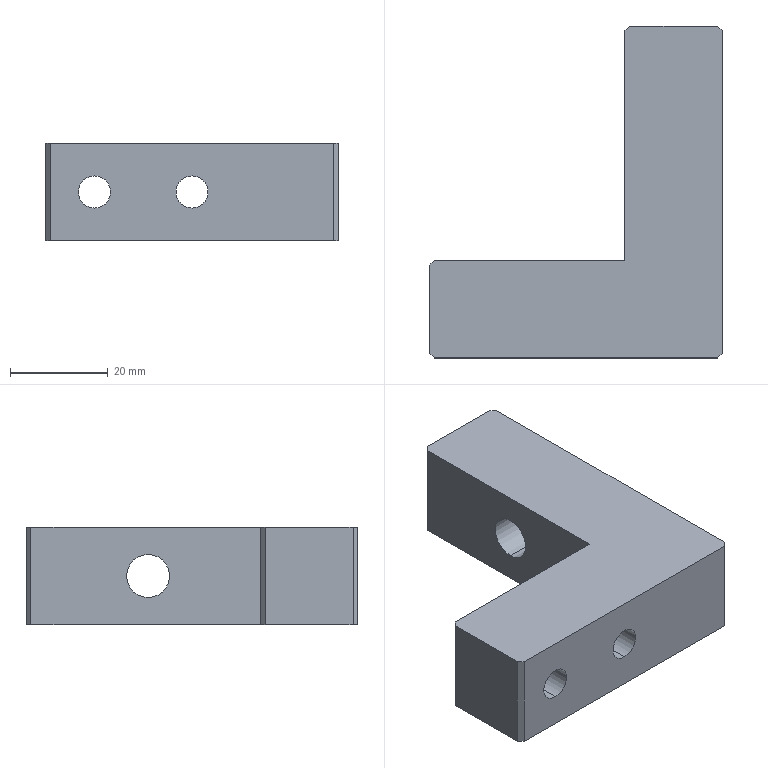Part | SolidWorks | features HoleWzd 2, Chamfer 1, Extrusion 1 | 1 solid | 25 faces | box 60 x 68 x 20 mm | volume 39349 mm3 | plane 15 | cylinder 10 | commonest cylinder face diameters 6.6 x4 11 x4 8.8 x2
STEP:
#1=CARTESIAN_POINT('',(-3.564,-15.126,4.5));
#2=VERTEX_POINT('',#1);
#3=CARTESIAN_POINT('',(-3.564,-15.126,15.5));
#4=VERTEX_POINT('',#3);
#5=CARTESIAN_POINT('',(-3.564,-15.126,10.));
#6=DIRECTION('',(0.,1.,0.));
#7=DIRECTION('',(0.,0.,1.));
#8=AXIS2_PLACEMENT_3D('',#5,#6,#7);
#9=CIRCLE('',#8,5.5);
#10=EDGE_CURVE('',#2,#4,#9,.T.);
#11=ORIENTED_EDGE('',*,*,#10,.F.);
#12=CARTESIAN_POINT('',(-3.564,-5.126,4.5));
#13=VERTEX_POINT('',#12);
#14=CARTESIAN_POINT('',(-3.564,-5.126,4.5));
#15=DIRECTION('',(0.,1.,0.));
#16=VECTOR('',#15,1000.);
#17=LINE('',#14,#16);
#18=EDGE_CURVE('',#2,#13,#17,.T.);
#19=ORIENTED_EDGE('',*,*,#18,.T.);
#20=CARTESIAN_POINT('',(-3.564,-5.126,15.5));
#21=VERTEX_POINT('',#20);
#22=CARTESIAN_POINT('',(-3.564,-5.126,10.));
#23=DIRECTION('',(0.,1.,0.));
#24=DIRECTION('',(0.,0.,1.));
#25=AXIS2_PLACEMENT_3D('',#22,#23,#24);
#26=CIRCLE('',#25,5.5);
#27=EDGE_CURVE('',#13,#21,#26,.T.);
#28=ORIENTED_EDGE('',*,*,#27,.T.);
#29=CARTESIAN_POINT('',(-3.564,-5.126,15.5));
#30=DIRECTION('',(0.,1.,0.));
#31=VECTOR('',#30,1000.);
#32=LINE('',#29,#31);
#33=EDGE_CURVE('',#4,#21,#32,.T.);
#34=ORIENTED_EDGE('',*,*,#33,.F.);
#35=EDGE_LOOP('',(#11,#19,#28,#34));
#36=FACE_OUTER_BOUND('',#35,.T.);
#37=CARTESIAN_POINT('',(-3.564,-5.126,10.));
#38=DIRECTION('',(0.,1.,0.));
#39=DIRECTION('',(0.,0.,1.));
#40=AXIS2_PLACEMENT_3D('',#37,#38,#39);
#41=CYLINDRICAL_SURFACE('',#40,5.5);
#42=ADVANCED_FACE('',(#36),#41,.F.);
#43=CARTESIAN_POINT('',(-3.564,-25.126,6.7));
#44=VERTEX_POINT('',#43);
#45=CARTESIAN_POINT('',(-3.564,-25.126,13.3));
#46=VERTEX_POINT('',#45);
#47=CARTESIAN_POINT('',(-3.564,-25.126,10.));
#48=DIRECTION('',(0.,1.,0.));
#49=DIRECTION('',(0.,0.,1.));
#50=AXIS2_PLACEMENT_3D('',#47,#48,#49);
#51=CIRCLE('',#50,3.3);
#52=EDGE_CURVE('',#44,#46,#51,.T.);
#53=ORIENTED_EDGE('',*,*,#52,.F.);
#54=CARTESIAN_POINT('',(-3.564,-15.126,6.7));
#55=VERTEX_POINT('',#54);
#56=CARTESIAN_POINT('',(-3.564,-5.126,6.7));
#57=DIRECTION('',(0.,1.,0.));
#58=VECTOR('',#57,1000.);
#59=LINE('',#56,#58);
#60=EDGE_CURVE('',#44,#55,#59,.T.);
#61=ORIENTED_EDGE('',*,*,#60,.T.);
#62=CARTESIAN_POINT('',(-3.564,-15.126,13.3));
#63=VERTEX_POINT('',#62);
#64=CARTESIAN_POINT('',(-3.564,-15.126,10.));
#65=DIRECTION('',(0.,1.,0.));
#66=DIRECTION('',(0.,0.,1.));
#67=AXIS2_PLACEMENT_3D('',#64,#65,#66);
#68=CIRCLE('',#67,3.3);
#69=EDGE_CURVE('',#55,#63,#68,.T.);
#70=ORIENTED_EDGE('',*,*,#69,.T.);
#71=CARTESIAN_POINT('',(-3.564,-5.126,13.3));
#72=DIRECTION('',(0.,1.,0.));
#73=VECTOR('',#72,1000.);
#74=LINE('',#71,#73);
#75=EDGE_CURVE('',#46,#63,#74,.T.);
#76=ORIENTED_EDGE('',*,*,#75,.F.);
#77=EDGE_LOOP('',(#53,#61,#70,#76));
#78=FACE_OUTER_BOUND('',#77,.T.);
#79=CARTESIAN_POINT('',(-3.564,-5.126,10.));
#80=DIRECTION('',(0.,1.,0.));
#81=DIRECTION('',(0.,0.,1.));
#82=AXIS2_PLACEMENT_3D('',#79,#80,#81);
#83=CYLINDRICAL_SURFACE('',#82,3.3);
#84=ADVANCED_FACE('',(#78),#83,.F.);
#85=CARTESIAN_POINT('',(-23.564,-15.126,4.5));
#86=VERTEX_POINT('',#85);
#87=CARTESIAN_POINT('',(-23.564,-15.126,15.5));
#88=VERTEX_POINT('',#87);
#89=CARTESIAN_POINT('',(-23.564,-15.126,10.));
#90=DIRECTION('',(0.,1.,0.));
#91=DIRECTION('',(0.,0.,1.));
#92=AXIS2_PLACEMENT_3D('',#89,#90,#91);
#93=CIRCLE('',#92,5.5);
#94=EDGE_CURVE('',#86,#88,#93,.T.);
#95=ORIENTED_EDGE('',*,*,#94,.F.);
#96=CARTESIAN_POINT('',(-23.564,-5.126,4.5));
#97=VERTEX_POINT('',#96);
#98=CARTESIAN_POINT('',(-23.564,-5.126,4.5));
#99=DIRECTION('',(0.,1.,0.));
#100=VECTOR('',#99,1000.);
#101=LINE('',#98,#100);
#102=EDGE_CURVE('',#86,#97,#101,.T.);
#103=ORIENTED_EDGE('',*,*,#102,.T.);
#104=CARTESIAN_POINT('',(-23.564,-5.126,15.5));
#105=VERTEX_POINT('',#104);
#106=CARTESIAN_POINT('',(-23.564,-5.126,10.));
#107=DIRECTION('',(0.,1.,0.));
#108=DIRECTION('',(0.,0.,1.));
#109=AXIS2_PLACEMENT_3D('',#106,#107,#108);
#110=CIRCLE('',#109,5.5);
#111=EDGE_CURVE('',#97,#105,#110,.T.);
#112=ORIENTED_EDGE('',*,*,#111,.T.);
#113=CARTESIAN_POINT('',(-23.564,-5.126,15.5));
#114=DIRECTION('',(0.,1.,0.));
#115=VECTOR('',#114,1000.);
#116=LINE('',#113,#115);
#117=EDGE_CURVE('',#88,#105,#116,.T.);
#118=ORIENTED_EDGE('',*,*,#117,.F.);
#119=EDGE_LOOP('',(#95,#103,#112,#118));
#120=FACE_OUTER_BOUND('',#119,.T.);
#121=CARTESIAN_POINT('',(-23.564,-5.126,10.));
#122=DIRECTION('',(0.,1.,0.));
#123=DIRECTION('',(0.,0.,1.));
#124=AXIS2_PLACEMENT_3D('',#121,#122,#123);
#125=CYLINDRICAL_SURFACE('',#124,5.5);
#126=ADVANCED_FACE('',(#120),#125,.F.);
#127=CARTESIAN_POINT('',(-23.564,-25.126,6.7));
#128=VERTEX_POINT('',#127);
#129=CARTESIAN_POINT('',(-23.564,-25.126,13.3));
#130=VERTEX_POINT('',#129);
#131=CARTESIAN_POINT('',(-23.564,-25.126,10.));
#132=DIRECTION('',(0.,1.,0.));
#133=DIRECTION('',(0.,0.,1.));
#134=AXIS2_PLACEMENT_3D('',#131,#132,#133);
#135=CIRCLE('',#134,3.3);
#136=EDGE_CURVE('',#128,#130,#135,.T.);
#137=ORIENTED_EDGE('',*,*,#136,.F.);
#138=CARTESIAN_POINT('',(-23.564,-15.126,6.7));
#139=VERTEX_POINT('',#138);
#140=CARTESIAN_POINT('',(-23.564,-5.126,6.7));
#141=DIRECTION('',(0.,1.,0.));
#142=VECTOR('',#141,1000.);
#143=LINE('',#140,#142);
#144=EDGE_CURVE('',#128,#139,#143,.T.);
#145=ORIENTED_EDGE('',*,*,#144,.T.);
#146=CARTESIAN_POINT('',(-23.564,-15.126,13.3));
#147=VERTEX_POINT('',#146);
#148=CARTESIAN_POINT('',(-23.564,-15.126,10.));
#149=DIRECTION('',(0.,1.,0.));
#150=DIRECTION('',(0.,0.,1.));
#151=AXIS2_PLACEMENT_3D('',#148,#149,#150);
#152=CIRCLE('',#151,3.3);
#153=EDGE_CURVE('',#139,#147,#152,.T.);
#154=ORIENTED_EDGE('',*,*,#153,.T.);
#155=CARTESIAN_POINT('',(-23.564,-5.126,13.3));
#156=DIRECTION('',(0.,1.,0.));
#157=VECTOR('',#156,1000.);
#158=LINE('',#155,#157);
#159=EDGE_CURVE('',#130,#147,#158,.T.);
#160=ORIENTED_EDGE('',*,*,#159,.F.);
#161=EDGE_LOOP('',(#137,#145,#154,#160));
#162=FACE_OUTER_BOUND('',#161,.T.);
#163=CARTESIAN_POINT('',(-23.564,-5.126,10.));
#164=DIRECTION('',(0.,1.,0.));
#165=DIRECTION('',(0.,0.,1.));
#166=AXIS2_PLACEMENT_3D('',#163,#164,#165);
#167=CYLINDRICAL_SURFACE('',#166,3.3);
#168=ADVANCED_FACE('',(#162),#167,.F.);
#169=CARTESIAN_POINT('',(26.436,17.874,5.6));
#170=VERTEX_POINT('',#169);
#171=CARTESIAN_POINT('',(26.436,17.874,14.4));
#172=VERTEX_POINT('',#171);
#173=CARTESIAN_POINT('',(26.436,17.874,10.));
#174=DIRECTION('',(-1.,0.,0.));
#175=DIRECTION('',(0.,0.,1.));
#176=AXIS2_PLACEMENT_3D('',#173,#174,#175);
#177=CIRCLE('',#176,4.4);
#178=EDGE_CURVE('',#170,#172,#177,.T.);
#179=ORIENTED_EDGE('',*,*,#178,.F.);
#180=CARTESIAN_POINT('',(6.436,17.874,5.6));
#181=VERTEX_POINT('',#180);
#182=CARTESIAN_POINT('',(6.436,17.874,5.6));
#183=DIRECTION('',(-1.,0.,0.));
#184=VECTOR('',#183,1000.);
#185=LINE('',#182,#184);
#186=EDGE_CURVE('',#170,#181,#185,.T.);
#187=ORIENTED_EDGE('',*,*,#186,.T.);
#188=CARTESIAN_POINT('',(6.436,17.874,14.4));
#189=VERTEX_POINT('',#188);
#190=CARTESIAN_POINT('',(6.436,17.874,10.));
#191=DIRECTION('',(-1.,0.,0.));
#192=DIRECTION('',(0.,0.,1.));
#193=AXIS2_PLACEMENT_3D('',#190,#191,#192);
#194=CIRCLE('',#193,4.4);
#195=EDGE_CURVE('',#181,#189,#194,.T.);
#196=ORIENTED_EDGE('',*,*,#195,.T.);
#197=CARTESIAN_POINT('',(6.436,17.874,14.4));
#198=DIRECTION('',(-1.,0.,0.));
#199=VECTOR('',#198,1000.);
#200=LINE('',#197,#199);
#201=EDGE_CURVE('',#172,#189,#200,.T.);
#202=ORIENTED_EDGE('',*,*,#201,.F.);
#203=EDGE_LOOP('',(#179,#187,#196,#202));
#204=FACE_OUTER_BOUND('',#203,.T.);
#205=CARTESIAN_POINT('',(6.436,17.874,10.));
#206=DIRECTION('',(-1.,0.,0.));
#207=DIRECTION('',(0.,0.,1.));
#208=AXIS2_PLACEMENT_3D('',#205,#206,#207);
#209=CYLINDRICAL_SURFACE('',#208,4.4);
#210=ADVANCED_FACE('',(#204),#209,.F.);
#211=CARTESIAN_POINT('',(25.436,42.874,0.));
#212=VERTEX_POINT('',#211);
#213=CARTESIAN_POINT('',(7.436,42.874,0.));
#214=VERTEX_POINT('',#213);
#215=CARTESIAN_POINT('',(26.436,42.874,0.));
#216=DIRECTION('',(-1.,0.,0.));
#217=VECTOR('',#216,1000.);
#218=LINE('',#215,#217);
#219=EDGE_CURVE('',#212,#214,#218,.T.);
#220=ORIENTED_EDGE('',*,*,#219,.T.);
#221=CARTESIAN_POINT('',(7.436,42.874,20.));
#222=VERTEX_POINT('',#221);
#223=CARTESIAN_POINT('',(7.436,42.874,20.));
#224=DIRECTION('',(0.,0.,1.));
#225=VECTOR('',#224,1000.);
#226=LINE('',#223,#225);
#227=EDGE_CURVE('',#214,#222,#226,.T.);
#228=ORIENTED_EDGE('',*,*,#227,.T.);
#229=CARTESIAN_POINT('',(25.436,42.874,20.));
#230=VERTEX_POINT('',#229);
#231=CARTESIAN_POINT('',(26.436,42.874,20.));
#232=DIRECTION('',(-1.,0.,0.));
#233=VECTOR('',#232,1000.);
#234=LINE('',#231,#233);
#235=EDGE_CURVE('',#230,#222,#234,.T.);
#236=ORIENTED_EDGE('',*,*,#235,.F.);
#237=CARTESIAN_POINT('',(25.436,42.874,20.));
#238=DIRECTION('',(0.,0.,-1.));
#239=VECTOR('',#238,1000.);
#240=LINE('',#237,#239);
#241=EDGE_CURVE('',#230,#212,#240,.T.);
#242=ORIENTED_EDGE('',*,*,#241,.T.);
#243=EDGE_LOOP('',(#220,#228,#236,#242));
#244=FACE_OUTER_BOUND('',#243,.T.);
#245=CARTESIAN_POINT('',(26.436,42.874,20.));
#246=DIRECTION('',(0.,-1.,0.));
#247=DIRECTION('',(0.,0.,-1.));
#248=AXIS2_PLACEMENT_3D('',#245,#246,#247);
#249=PLANE('',#248);
#250=ADVANCED_FACE('',(#244),#249,.F.);
#251=CARTESIAN_POINT('',(6.436,17.874,10.));
#252=DIRECTION('',(-1.,0.,0.));
#253=DIRECTION('',(0.,0.,1.));
#254=AXIS2_PLACEMENT_3D('',#251,#252,#253);
#255=CIRCLE('',#254,4.4);
#256=EDGE_CURVE('',#189,#181,#255,.T.);
#257=ORIENTED_EDGE('',*,*,#256,.F.);
#258=ORIENTED_EDGE('',*,*,#195,.F.);
#259=EDGE_LOOP('',(#257,#258));
#260=FACE_BOUND('',#259,.T.);
#261=CARTESIAN_POINT('',(6.436,41.874,20.));
#262=VERTEX_POINT('',#261);
#263=CARTESIAN_POINT('',(6.436,-5.126,20.));
#264=VERTEX_POINT('',#263);
#265=CARTESIAN_POINT('',(6.436,42.874,20.));
#266=DIRECTION('',(0.,-1.,0.));
#267=VECTOR('',#266,1000.);
#268=LINE('',#265,#267);
#269=EDGE_CURVE('',#262,#264,#268,.T.);
#270=ORIENTED_EDGE('',*,*,#269,.F.);
#271=CARTESIAN_POINT('',(6.436,41.874,0.));
#272=VERTEX_POINT('',#271);
#273=CARTESIAN_POINT('',(6.436,41.874,20.));
#274=DIRECTION('',(0.,0.,-1.));
#275=VECTOR('',#274,1000.);
#276=LINE('',#273,#275);
#277=EDGE_CURVE('',#262,#272,#276,.T.);
#278=ORIENTED_EDGE('',*,*,#277,.T.);
#279=CARTESIAN_POINT('',(6.436,-5.126,0.));
#280=VERTEX_POINT('',#279);
#281=CARTESIAN_POINT('',(6.436,42.874,0.));
#282=DIRECTION('',(0.,-1.,0.));
#283=VECTOR('',#282,1000.);
#284=LINE('',#281,#283);
#285=EDGE_CURVE('',#272,#280,#284,.T.);
#286=ORIENTED_EDGE('',*,*,#285,.T.);
#287=CARTESIAN_POINT('',(6.436,-5.126,20.));
#288=DIRECTION('',(0.,0.,-1.));
#289=VECTOR('',#288,1000.);
#290=LINE('',#287,#289);
#291=EDGE_CURVE('',#264,#280,#290,.T.);
#292=ORIENTED_EDGE('',*,*,#291,.F.);
#293=EDGE_LOOP('',(#270,#278,#286,#292));
#294=FACE_OUTER_BOUND('',#293,.T.);
#295=CARTESIAN_POINT('',(6.436,42.874,20.));
#296=DIRECTION('',(1.,0.,0.));
#297=DIRECTION('',(0.,1.,0.));
#298=AXIS2_PLACEMENT_3D('',#295,#296,#297);
#299=PLANE('',#298);
#300=ADVANCED_FACE('',(#260,#294),#299,.F.);
#301=CARTESIAN_POINT('',(-3.564,-5.126,10.));
#302=DIRECTION('',(0.,1.,0.));
#303=DIRECTION('',(0.,0.,1.));
#304=AXIS2_PLACEMENT_3D('',#301,#302,#303);
#305=CIRCLE('',#304,5.5);
#306=EDGE_CURVE('',#21,#13,#305,.T.);
#307=ORIENTED_EDGE('',*,*,#306,.F.);
#308=ORIENTED_EDGE('',*,*,#27,.F.);
#309=EDGE_LOOP('',(#307,#308));
#310=FACE_BOUND('',#309,.T.);
#311=CARTESIAN_POINT('',(-23.564,-5.126,10.));
#312=DIRECTION('',(0.,1.,0.));
#313=DIRECTION('',(0.,0.,1.));
#314=AXIS2_PLACEMENT_3D('',#311,#312,#313);
#315=CIRCLE('',#314,5.5);
#316=EDGE_CURVE('',#105,#97,#315,.T.);
#317=ORIENTED_EDGE('',*,*,#316,.F.);
#318=ORIENTED_EDGE('',*,*,#111,.F.);
#319=EDGE_LOOP('',(#317,#318));
#320=FACE_BOUND('',#319,.T.);
#321=CARTESIAN_POINT('',(-32.564,-5.126,0.));
#322=VERTEX_POINT('',#321);
#323=CARTESIAN_POINT('',(6.436,-5.126,0.));
#324=DIRECTION('',(-1.,0.,0.));
#325=VECTOR('',#324,1000.);
#326=LINE('',#323,#325);
#327=EDGE_CURVE('',#280,#322,#326,.T.);
#328=ORIENTED_EDGE('',*,*,#327,.T.);
#329=CARTESIAN_POINT('',(-32.564,-5.126,20.));
#330=VERTEX_POINT('',#329);
#331=CARTESIAN_POINT('',(-32.564,-5.126,20.));
#332=DIRECTION('',(0.,0.,1.));
#333=VECTOR('',#332,1000.);
#334=LINE('',#331,#333);
#335=EDGE_CURVE('',#322,#330,#334,.T.);
#336=ORIENTED_EDGE('',*,*,#335,.T.);
#337=CARTESIAN_POINT('',(6.436,-5.126,20.));
#338=DIRECTION('',(-1.,0.,0.));
#339=VECTOR('',#338,1000.);
#340=LINE('',#337,#339);
#341=EDGE_CURVE('',#264,#330,#340,.T.);
#342=ORIENTED_EDGE('',*,*,#341,.F.);
#343=ORIENTED_EDGE('',*,*,#291,.T.);
#344=EDGE_LOOP('',(#328,#336,#342,#343));
#345=FACE_OUTER_BOUND('',#344,.T.);
#346=CARTESIAN_POINT('',(6.436,-5.126,20.));
#347=DIRECTION('',(0.,-1.,0.));
#348=DIRECTION('',(1.,0.,0.));
#349=AXIS2_PLACEMENT_3D('',#346,#347,#348);
#350=PLANE('',#349);
#351=ADVANCED_FACE('',(#310,#320,#345),#350,.F.);
#352=CARTESIAN_POINT('',(-33.564,-6.126,0.));
#353=VERTEX_POINT('',#352);
#354=CARTESIAN_POINT('',(-33.564,-24.126,0.));
#355=VERTEX_POINT('',#354);
#356=CARTESIAN_POINT('',(-33.564,-5.126,0.));
#357=DIRECTION('',(0.,-1.,0.));
#358=VECTOR('',#357,1000.);
#359=LINE('',#356,#358);
#360=EDGE_CURVE('',#353,#355,#359,.T.);
#361=ORIENTED_EDGE('',*,*,#360,.T.);
#362=CARTESIAN_POINT('',(-33.564,-24.126,20.));
#363=VERTEX_POINT('',#362);
#364=CARTESIAN_POINT('',(-33.564,-24.126,20.));
#365=DIRECTION('',(0.,0.,1.));
#366=VECTOR('',#365,1000.);
#367=LINE('',#364,#366);
#368=EDGE_CURVE('',#355,#363,#367,.T.);
#369=ORIENTED_EDGE('',*,*,#368,.T.);
#370=CARTESIAN_POINT('',(-33.564,-6.126,20.));
#371=VERTEX_POINT('',#370);
#372=CARTESIAN_POINT('',(-33.564,-5.126,20.));
#373=DIRECTION('',(0.,-1.,0.));
#374=VECTOR('',#373,1000.);
#375=LINE('',#372,#374);
#376=EDGE_CURVE('',#371,#363,#375,.T.);
#377=ORIENTED_EDGE('',*,*,#376,.F.);
#378=CARTESIAN_POINT('',(-33.564,-6.126,20.));
#379=DIRECTION('',(0.,0.,-1.));
#380=VECTOR('',#379,1000.);
#381=LINE('',#378,#380);
#382=EDGE_CURVE('',#371,#353,#381,.T.);
#383=ORIENTED_EDGE('',*,*,#382,.T.);
#384=EDGE_LOOP('',(#361,#369,#377,#383));
#385=FACE_OUTER_BOUND('',#384,.T.);
#386=CARTESIAN_POINT('',(-33.564,-5.126,20.));
#387=DIRECTION('',(1.,0.,0.));
#388=DIRECTION('',(0.,1.,0.));
#389=AXIS2_PLACEMENT_3D('',#386,#387,#388);
#390=PLANE('',#389);
#391=ADVANCED_FACE('',(#385),#390,.F.);
#392=CARTESIAN_POINT('',(-3.564,-25.126,10.));
#393=DIRECTION('',(0.,1.,0.));
#394=DIRECTION('',(0.,0.,1.));
#395=AXIS2_PLACEMENT_3D('',#392,#393,#394);
#396=CIRCLE('',#395,3.3);
#397=EDGE_CURVE('',#46,#44,#396,.T.);
#398=ORIENTED_EDGE('',*,*,#397,.T.);
#399=ORIENTED_EDGE('',*,*,#52,.T.);
#400=EDGE_LOOP('',(#398,#399));
#401=FACE_BOUND('',#400,.T.);
#402=CARTESIAN_POINT('',(-23.564,-25.126,10.));
#403=DIRECTION('',(0.,1.,0.));
#404=DIRECTION('',(0.,0.,1.));
#405=AXIS2_PLACEMENT_3D('',#402,#403,#404);
#406=CIRCLE('',#405,3.3);
#407=EDGE_CURVE('',#130,#128,#406,.T.);
#408=ORIENTED_EDGE('',*,*,#407,.T.);
#409=ORIENTED_EDGE('',*,*,#136,.T.);
#410=EDGE_LOOP('',(#408,#409));
#411=FACE_BOUND('',#410,.T.);
#412=CARTESIAN_POINT('',(-32.564,-25.126,0.));
#413=VERTEX_POINT('',#412);
#414=CARTESIAN_POINT('',(25.436,-25.126,0.));
#415=VERTEX_POINT('',#414);
#416=CARTESIAN_POINT('',(-33.564,-25.126,0.));
#417=DIRECTION('',(1.,0.,0.));
#418=VECTOR('',#417,1000.);
#419=LINE('',#416,#418);
#420=EDGE_CURVE('',#413,#415,#419,.T.);
#421=ORIENTED_EDGE('',*,*,#420,.T.);
#422=CARTESIAN_POINT('',(25.436,-25.126,20.));
#423=VERTEX_POINT('',#422);
#424=CARTESIAN_POINT('',(25.436,-25.126,20.));
#425=DIRECTION('',(0.,0.,1.));
#426=VECTOR('',#425,1000.);
#427=LINE('',#424,#426);
#428=EDGE_CURVE('',#415,#423,#427,.T.);
#429=ORIENTED_EDGE('',*,*,#428,.T.);
#430=CARTESIAN_POINT('',(-32.564,-25.126,20.));
#431=VERTEX_POINT('',#430);
#432=CARTESIAN_POINT('',(-33.564,-25.126,20.));
#433=DIRECTION('',(1.,0.,0.));
#434=VECTOR('',#433,1000.);
#435=LINE('',#432,#434);
#436=EDGE_CURVE('',#431,#423,#435,.T.);
#437=ORIENTED_EDGE('',*,*,#436,.F.);
#438=CARTESIAN_POINT('',(-32.564,-25.126,20.));
#439=DIRECTION('',(0.,0.,-1.));
#440=VECTOR('',#439,1000.);
#441=LINE('',#438,#440);
#442=EDGE_CURVE('',#431,#413,#441,.T.);
#443=ORIENTED_EDGE('',*,*,#442,.T.);
#444=EDGE_LOOP('',(#421,#429,#437,#443));
#445=FACE_OUTER_BOUND('',#444,.T.);
#446=CARTESIAN_POINT('',(-33.564,-25.126,20.));
#447=DIRECTION('',(0.,1.,0.));
#448=DIRECTION('',(0.,0.,1.));
#449=AXIS2_PLACEMENT_3D('',#446,#447,#448);
#450=PLANE('',#449);
#451=ADVANCED_FACE('',(#401,#411,#445),#450,.F.);
#452=CARTESIAN_POINT('',(26.436,17.874,10.));
#453=DIRECTION('',(-1.,0.,0.));
#454=DIRECTION('',(0.,0.,1.));
#455=AXIS2_PLACEMENT_3D('',#452,#453,#454);
#456=CIRCLE('',#455,4.4);
#457=EDGE_CURVE('',#172,#170,#456,.T.);
#458=ORIENTED_EDGE('',*,*,#457,.T.);
#459=ORIENTED_EDGE('',*,*,#178,.T.);
#460=EDGE_LOOP('',(#458,#459));
#461=FACE_BOUND('',#460,.T.);
#462=CARTESIAN_POINT('',(26.436,-24.126,20.));
#463=VERTEX_POINT('',#462);
#464=CARTESIAN_POINT('',(26.436,41.874,20.));
#465=VERTEX_POINT('',#464);
#466=CARTESIAN_POINT('',(26.436,-25.126,20.));
#467=DIRECTION('',(0.,1.,0.));
#468=VECTOR('',#467,1000.);
#469=LINE('',#466,#468);
#470=EDGE_CURVE('',#463,#465,#469,.T.);
#471=ORIENTED_EDGE('',*,*,#470,.F.);
#472=CARTESIAN_POINT('',(26.436,-24.126,0.));
#473=VERTEX_POINT('',#472);
#474=CARTESIAN_POINT('',(26.436,-24.126,20.));
#475=DIRECTION('',(0.,0.,-1.));
#476=VECTOR('',#475,1000.);
#477=LINE('',#474,#476);
#478=EDGE_CURVE('',#463,#473,#477,.T.);
#479=ORIENTED_EDGE('',*,*,#478,.T.);
#480=CARTESIAN_POINT('',(26.436,41.874,0.));
#481=VERTEX_POINT('',#480);
#482=CARTESIAN_POINT('',(26.436,-25.126,0.));
#483=DIRECTION('',(0.,1.,0.));
#484=VECTOR('',#483,1000.);
#485=LINE('',#482,#484);
#486=EDGE_CURVE('',#473,#481,#485,.T.);
#487=ORIENTED_EDGE('',*,*,#486,.T.);
#488=CARTESIAN_POINT('',(26.436,41.874,20.));
#489=DIRECTION('',(0.,0.,1.));
#490=VECTOR('',#489,1000.);
#491=LINE('',#488,#490);
#492=EDGE_CURVE('',#481,#465,#491,.T.);
#493=ORIENTED_EDGE('',*,*,#492,.T.);
#494=EDGE_LOOP('',(#471,#479,#487,#493));
#495=FACE_OUTER_BOUND('',#494,.T.);
#496=CARTESIAN_POINT('',(26.436,-25.126,20.));
#497=DIRECTION('',(-1.,0.,0.));
#498=DIRECTION('',(0.,0.,1.));
#499=AXIS2_PLACEMENT_3D('',#496,#497,#498);
#500=PLANE('',#499);
#501=ADVANCED_FACE('',(#461,#495),#500,.F.);
#502=ORIENTED_EDGE('',*,*,#436,.T.);
#503=CARTESIAN_POINT('',(25.281,-25.281,20.));
#504=DIRECTION('',(0.7071,0.7071,0.));
#505=VECTOR('',#504,1000.);
#506=LINE('',#503,#505);
#507=EDGE_CURVE('',#423,#463,#506,.T.);
#508=ORIENTED_EDGE('',*,*,#507,.T.);
#509=ORIENTED_EDGE('',*,*,#470,.T.);
#510=CARTESIAN_POINT('',(34.155,34.155,20.));
#511=DIRECTION('',(-0.7071,0.7071,0.));
#512=VECTOR('',#511,1000.);
#513=LINE('',#510,#512);
#514=EDGE_CURVE('',#465,#230,#513,.T.);
#515=ORIENTED_EDGE('',*,*,#514,.T.);
#516=ORIENTED_EDGE('',*,*,#235,.T.);
#517=CARTESIAN_POINT('',(-17.719,17.719,20.));
#518=DIRECTION('',(-0.7071,-0.7071,0.));
#519=VECTOR('',#518,1000.);
#520=LINE('',#517,#519);
#521=EDGE_CURVE('',#222,#262,#520,.T.);
#522=ORIENTED_EDGE('',*,*,#521,.T.);
#523=ORIENTED_EDGE('',*,*,#269,.T.);
#524=ORIENTED_EDGE('',*,*,#341,.T.);
#525=CARTESIAN_POINT('',(-13.719,13.719,20.));
#526=DIRECTION('',(-0.7071,-0.7071,0.));
#527=VECTOR('',#526,1000.);
#528=LINE('',#525,#527);
#529=EDGE_CURVE('',#330,#371,#528,.T.);
#530=ORIENTED_EDGE('',*,*,#529,.T.);
#531=ORIENTED_EDGE('',*,*,#376,.T.);
#532=CARTESIAN_POINT('',(-28.845,-28.845,20.));
#533=DIRECTION('',(0.7071,-0.7071,0.));
#534=VECTOR('',#533,1000.);
#535=LINE('',#532,#534);
#536=EDGE_CURVE('',#363,#431,#535,.T.);
#537=ORIENTED_EDGE('',*,*,#536,.T.);
#538=EDGE_LOOP('',(#502,#508,#509,#515,#516,#522,#523,#524,#530,#531,#537));
#539=FACE_OUTER_BOUND('',#538,.T.);
#540=CARTESIAN_POINT('',(0.,0.,20.));
#541=DIRECTION('',(0.,0.,1.));
#542=DIRECTION('',(1.,0.,0.));
#543=AXIS2_PLACEMENT_3D('',#540,#541,#542);
#544=PLANE('',#543);
#545=ADVANCED_FACE('',(#539),#544,.T.);
#546=ORIENTED_EDGE('',*,*,#486,.F.);
#547=CARTESIAN_POINT('',(26.436,-24.126,0.));
#548=DIRECTION('',(-0.7071,-0.7071,0.));
#549=VECTOR('',#548,1000.);
#550=LINE('',#547,#549);
#551=EDGE_CURVE('',#473,#415,#550,.T.);
#552=ORIENTED_EDGE('',*,*,#551,.T.);
#553=ORIENTED_EDGE('',*,*,#420,.F.);
#554=CARTESIAN_POINT('',(-32.564,-25.126,0.));
#555=DIRECTION('',(-0.7071,0.7071,0.));
#556=VECTOR('',#555,1000.);
#557=LINE('',#554,#556);
#558=EDGE_CURVE('',#413,#355,#557,.T.);
#559=ORIENTED_EDGE('',*,*,#558,.T.);
#560=ORIENTED_EDGE('',*,*,#360,.F.);
#561=CARTESIAN_POINT('',(-33.564,-6.126,0.));
#562=DIRECTION('',(0.7071,0.7071,0.));
#563=VECTOR('',#562,1000.);
#564=LINE('',#561,#563);
#565=EDGE_CURVE('',#353,#322,#564,.T.);
#566=ORIENTED_EDGE('',*,*,#565,.T.);
#567=ORIENTED_EDGE('',*,*,#327,.F.);
#568=ORIENTED_EDGE('',*,*,#285,.F.);
#569=CARTESIAN_POINT('',(6.436,41.874,0.));
#570=DIRECTION('',(0.7071,0.7071,0.));
#571=VECTOR('',#570,1000.);
#572=LINE('',#569,#571);
#573=EDGE_CURVE('',#272,#214,#572,.T.);
#574=ORIENTED_EDGE('',*,*,#573,.T.);
#575=ORIENTED_EDGE('',*,*,#219,.F.);
#576=CARTESIAN_POINT('',(25.436,42.874,0.));
#577=DIRECTION('',(0.7071,-0.7071,0.));
#578=VECTOR('',#577,1000.);
#579=LINE('',#576,#578);
#580=EDGE_CURVE('',#212,#481,#579,.T.);
#581=ORIENTED_EDGE('',*,*,#580,.T.);
#582=EDGE_LOOP('',(#546,#552,#553,#559,#560,#566,#567,#568,#574,#575,#581));
#583=FACE_OUTER_BOUND('',#582,.T.);
#584=CARTESIAN_POINT('',(0.,0.,0.));
#585=DIRECTION('',(0.,0.,1.));
#586=DIRECTION('',(1.,0.,0.));
#587=AXIS2_PLACEMENT_3D('',#584,#585,#586);
#588=PLANE('',#587);
#589=ADVANCED_FACE('',(#583),#588,.F.);
#590=ORIENTED_EDGE('',*,*,#186,.F.);
#591=ORIENTED_EDGE('',*,*,#457,.F.);
#592=ORIENTED_EDGE('',*,*,#201,.T.);
#593=ORIENTED_EDGE('',*,*,#256,.T.);
#594=EDGE_LOOP('',(#590,#591,#592,#593));
#595=FACE_OUTER_BOUND('',#594,.T.);
#596=CARTESIAN_POINT('',(6.436,17.874,10.));
#597=DIRECTION('',(-1.,0.,0.));
#598=DIRECTION('',(0.,0.,1.));
#599=AXIS2_PLACEMENT_3D('',#596,#597,#598);
#600=CYLINDRICAL_SURFACE('',#599,4.4);
#601=ADVANCED_FACE('',(#595),#600,.F.);
#602=ORIENTED_EDGE('',*,*,#144,.F.);
#603=ORIENTED_EDGE('',*,*,#407,.F.);
#604=ORIENTED_EDGE('',*,*,#159,.T.);
#605=CARTESIAN_POINT('',(-23.564,-15.126,10.));
#606=DIRECTION('',(0.,1.,0.));
#607=DIRECTION('',(0.,0.,1.));
#608=AXIS2_PLACEMENT_3D('',#605,#606,#607);
#609=CIRCLE('',#608,3.3);
#610=EDGE_CURVE('',#147,#139,#609,.T.);
#611=ORIENTED_EDGE('',*,*,#610,.T.);
#612=EDGE_LOOP('',(#602,#603,#604,#611));
#613=FACE_OUTER_BOUND('',#612,.T.);
#614=CARTESIAN_POINT('',(-23.564,-5.126,10.));
#615=DIRECTION('',(0.,1.,0.));
#616=DIRECTION('',(0.,0.,1.));
#617=AXIS2_PLACEMENT_3D('',#614,#615,#616);
#618=CYLINDRICAL_SURFACE('',#617,3.3);
#619=ADVANCED_FACE('',(#613),#618,.F.);
#620=ORIENTED_EDGE('',*,*,#610,.F.);
#621=ORIENTED_EDGE('',*,*,#153,.F.);
#622=EDGE_LOOP('',(#620,#621));
#623=FACE_BOUND('',#622,.T.);
#624=CARTESIAN_POINT('',(-23.564,-15.126,10.));
#625=DIRECTION('',(0.,1.,0.));
#626=DIRECTION('',(0.,0.,1.));
#627=AXIS2_PLACEMENT_3D('',#624,#625,#626);
#628=CIRCLE('',#627,5.5);
#629=EDGE_CURVE('',#88,#86,#628,.T.);
#630=ORIENTED_EDGE('',*,*,#629,.T.);
#631=ORIENTED_EDGE('',*,*,#94,.T.);
#632=EDGE_LOOP('',(#630,#631));
#633=FACE_OUTER_BOUND('',#632,.T.);
#634=CARTESIAN_POINT('',(-20.264,-15.126,10.));
#635=DIRECTION('',(0.,-1.,0.));
#636=DIRECTION('',(0.,0.,-1.));
#637=AXIS2_PLACEMENT_3D('',#634,#635,#636);
#638=PLANE('',#637);
#639=ADVANCED_FACE('',(#623,#633),#638,.F.);
#640=ORIENTED_EDGE('',*,*,#102,.F.);
#641=ORIENTED_EDGE('',*,*,#629,.F.);
#642=ORIENTED_EDGE('',*,*,#117,.T.);
#643=ORIENTED_EDGE('',*,*,#316,.T.);
#644=EDGE_LOOP('',(#640,#641,#642,#643));
#645=FACE_OUTER_BOUND('',#644,.T.);
#646=CARTESIAN_POINT('',(-23.564,-5.126,10.));
#647=DIRECTION('',(0.,1.,0.));
#648=DIRECTION('',(0.,0.,1.));
#649=AXIS2_PLACEMENT_3D('',#646,#647,#648);
#650=CYLINDRICAL_SURFACE('',#649,5.5);
#651=ADVANCED_FACE('',(#645),#650,.F.);
#652=ORIENTED_EDGE('',*,*,#60,.F.);
#653=ORIENTED_EDGE('',*,*,#397,.F.);
#654=ORIENTED_EDGE('',*,*,#75,.T.);
#655=CARTESIAN_POINT('',(-3.564,-15.126,10.));
#656=DIRECTION('',(0.,1.,0.));
#657=DIRECTION('',(0.,0.,1.));
#658=AXIS2_PLACEMENT_3D('',#655,#656,#657);
#659=CIRCLE('',#658,3.3);
#660=EDGE_CURVE('',#63,#55,#659,.T.);
#661=ORIENTED_EDGE('',*,*,#660,.T.);
#662=EDGE_LOOP('',(#652,#653,#654,#661));
#663=FACE_OUTER_BOUND('',#662,.T.);
#664=CARTESIAN_POINT('',(-3.564,-5.126,10.));
#665=DIRECTION('',(0.,1.,0.));
#666=DIRECTION('',(0.,0.,1.));
#667=AXIS2_PLACEMENT_3D('',#664,#665,#666);
#668=CYLINDRICAL_SURFACE('',#667,3.3);
#669=ADVANCED_FACE('',(#663),#668,.F.);
#670=ORIENTED_EDGE('',*,*,#660,.F.);
#671=ORIENTED_EDGE('',*,*,#69,.F.);
#672=EDGE_LOOP('',(#670,#671));
#673=FACE_BOUND('',#672,.T.);
#674=CARTESIAN_POINT('',(-3.564,-15.126,10.));
#675=DIRECTION('',(0.,1.,0.));
#676=DIRECTION('',(0.,0.,1.));
#677=AXIS2_PLACEMENT_3D('',#674,#675,#676);
#678=CIRCLE('',#677,5.5);
#679=EDGE_CURVE('',#4,#2,#678,.T.);
#680=ORIENTED_EDGE('',*,*,#679,.T.);
#681=ORIENTED_EDGE('',*,*,#10,.T.);
#682=EDGE_LOOP('',(#680,#681));
#683=FACE_OUTER_BOUND('',#682,.T.);
#684=CARTESIAN_POINT('',(-0.2639,-15.126,10.));
#685=DIRECTION('',(0.,-1.,0.));
#686=DIRECTION('',(0.,0.,-1.));
#687=AXIS2_PLACEMENT_3D('',#684,#685,#686);
#688=PLANE('',#687);
#689=ADVANCED_FACE('',(#673,#683),#688,.F.);
#690=ORIENTED_EDGE('',*,*,#18,.F.);
#691=ORIENTED_EDGE('',*,*,#679,.F.);
#692=ORIENTED_EDGE('',*,*,#33,.T.);
#693=ORIENTED_EDGE('',*,*,#306,.T.);
#694=EDGE_LOOP('',(#690,#691,#692,#693));
#695=FACE_OUTER_BOUND('',#694,.T.);
#696=CARTESIAN_POINT('',(-3.564,-5.126,10.));
#697=DIRECTION('',(0.,1.,0.));
#698=DIRECTION('',(0.,0.,1.));
#699=AXIS2_PLACEMENT_3D('',#696,#697,#698);
#700=CYLINDRICAL_SURFACE('',#699,5.5);
#701=ADVANCED_FACE('',(#695),#700,.F.);
#702=ORIENTED_EDGE('',*,*,#507,.F.);
#703=ORIENTED_EDGE('',*,*,#428,.F.);
#704=ORIENTED_EDGE('',*,*,#551,.F.);
#705=ORIENTED_EDGE('',*,*,#478,.F.);
#706=EDGE_LOOP('',(#702,#703,#704,#705));
#707=FACE_OUTER_BOUND('',#706,.T.);
#708=CARTESIAN_POINT('',(26.436,-24.126,20.));
#709=DIRECTION('',(-0.7071,0.7071,0.));
#710=DIRECTION('',(0.,0.,-1.));
#711=AXIS2_PLACEMENT_3D('',#708,#709,#710);
#712=PLANE('',#711);
#713=ADVANCED_FACE('',(#707),#712,.F.);
#714=ORIENTED_EDGE('',*,*,#536,.F.);
#715=ORIENTED_EDGE('',*,*,#368,.F.);
#716=ORIENTED_EDGE('',*,*,#558,.F.);
#717=ORIENTED_EDGE('',*,*,#442,.F.);
#718=EDGE_LOOP('',(#714,#715,#716,#717));
#719=FACE_OUTER_BOUND('',#718,.T.);
#720=CARTESIAN_POINT('',(-32.564,-25.126,20.));
#721=DIRECTION('',(0.7071,0.7071,0.));
#722=DIRECTION('',(0.,0.,-1.));
#723=AXIS2_PLACEMENT_3D('',#720,#721,#722);
#724=PLANE('',#723);
#725=ADVANCED_FACE('',(#719),#724,.F.);
#726=ORIENTED_EDGE('',*,*,#529,.F.);
#727=ORIENTED_EDGE('',*,*,#335,.F.);
#728=ORIENTED_EDGE('',*,*,#565,.F.);
#729=ORIENTED_EDGE('',*,*,#382,.F.);
#730=EDGE_LOOP('',(#726,#727,#728,#729));
#731=FACE_OUTER_BOUND('',#730,.T.);
#732=CARTESIAN_POINT('',(-33.564,-6.126,20.));
#733=DIRECTION('',(0.7071,-0.7071,0.));
#734=DIRECTION('',(0.,0.,-1.));
#735=AXIS2_PLACEMENT_3D('',#732,#733,#734);
#736=PLANE('',#735);
#737=ADVANCED_FACE('',(#731),#736,.F.);
#738=ORIENTED_EDGE('',*,*,#521,.F.);
#739=ORIENTED_EDGE('',*,*,#227,.F.);
#740=ORIENTED_EDGE('',*,*,#573,.F.);
#741=ORIENTED_EDGE('',*,*,#277,.F.);
#742=EDGE_LOOP('',(#738,#739,#740,#741));
#743=FACE_OUTER_BOUND('',#742,.T.);
#744=CARTESIAN_POINT('',(6.436,41.874,20.));
#745=DIRECTION('',(0.7071,-0.7071,0.));
#746=DIRECTION('',(0.,0.,-1.));
#747=AXIS2_PLACEMENT_3D('',#744,#745,#746);
#748=PLANE('',#747);
#749=ADVANCED_FACE('',(#743),#748,.F.);
#750=ORIENTED_EDGE('',*,*,#514,.F.);
#751=ORIENTED_EDGE('',*,*,#492,.F.);
#752=ORIENTED_EDGE('',*,*,#580,.F.);
#753=ORIENTED_EDGE('',*,*,#241,.F.);
#754=EDGE_LOOP('',(#750,#751,#752,#753));
#755=FACE_OUTER_BOUND('',#754,.T.);
#756=CARTESIAN_POINT('',(25.436,42.874,20.));
#757=DIRECTION('',(-0.7071,-0.7071,0.));
#758=DIRECTION('',(0.,0.,-1.));
#759=AXIS2_PLACEMENT_3D('',#756,#757,#758);
#760=PLANE('',#759);
#761=ADVANCED_FACE('',(#755),#760,.F.);
#762=CLOSED_SHELL('',(#42,#84,#126,#168,#210,#250,#300,#351,#391,#451,#501,#545,#589,#601,#619,#639,#651,#669,#689,#701,#713,#725,#737,#749,#761));
#763=MANIFOLD_SOLID_BREP('',#762);
#764=CARTESIAN_POINT('',(0.,0.,0.));
#765=DIRECTION('',(0.,0.,1.));
#766=DIRECTION('',(1.,0.,0.));
#767=AXIS2_PLACEMENT_3D('',#764,#765,#766);
#768=(LENGTH_UNIT()NAMED_UNIT(*)SI_UNIT(.MILLI.,.METRE.));
#769=UNCERTAINTY_MEASURE_WITH_UNIT(LENGTH_MEASURE(0.00001),#768,'','');
#770=(NAMED_UNIT(*)PLANE_ANGLE_UNIT()SI_UNIT($,.RADIAN.));
#771=(NAMED_UNIT(*)SI_UNIT($,.STERADIAN.)SOLID_ANGLE_UNIT());
#772=(GEOMETRIC_REPRESENTATION_CONTEXT(3)GLOBAL_UNCERTAINTY_ASSIGNED_CONTEXT((#769))GLOBAL_UNIT_ASSIGNED_CONTEXT((#768,#770,#771))REPRESENTATION_CONTEXT('',''));
#773=ADVANCED_BREP_SHAPE_REPRESENTATION('',(#763,#767),#772);